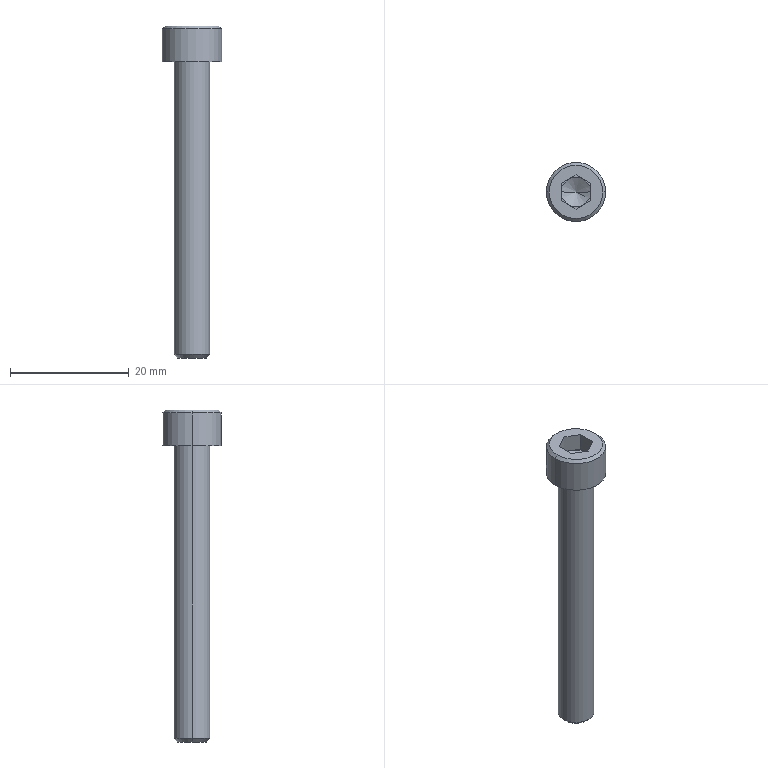Part | STEP file | 001-006-TAC01_M6_L50 | 1 solid | 25 faces | box 10 x 10 x 56 mm | volume 1803 mm3 | plane 15 | cone 6 | cylinder 4 | commonest cylinder face diameters 6 x2 10 x2